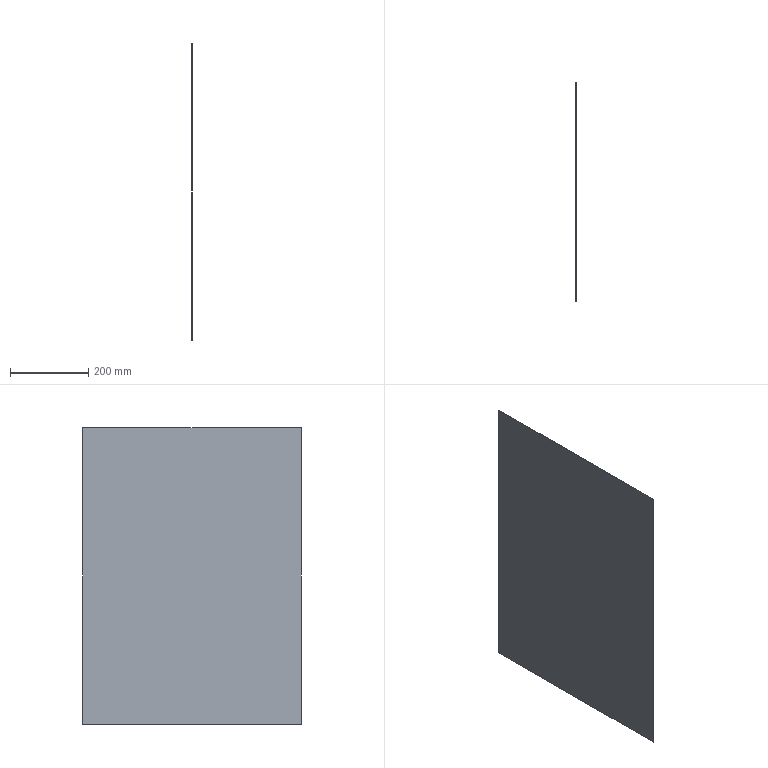Part | SolidWorks | 1 solid | 6 faces | box 1.5 x 560 x 759 mm | volume 637560 mm3 | plane 6
STEP:
#1=CARTESIAN_POINT('',(0.,280.,379.5));
#2=VERTEX_POINT('',#1);
#3=CARTESIAN_POINT('',(0.,-280.,379.5));
#4=VERTEX_POINT('',#3);
#5=CARTESIAN_POINT('',(0.,-280.,379.5));
#6=DIRECTION('',(0.,-1.,0.));
#7=VECTOR('',#6,1000.);
#8=LINE('',#5,#7);
#9=EDGE_CURVE('',#2,#4,#8,.T.);
#10=ORIENTED_EDGE('',*,*,#9,.F.);
#11=CARTESIAN_POINT('',(-1.5,280.,379.5));
#12=VERTEX_POINT('',#11);
#13=CARTESIAN_POINT('',(-1.5,280.,379.5));
#14=DIRECTION('',(1.,0.,0.));
#15=VECTOR('',#14,1000.);
#16=LINE('',#13,#15);
#17=EDGE_CURVE('',#12,#2,#16,.T.);
#18=ORIENTED_EDGE('',*,*,#17,.F.);
#19=CARTESIAN_POINT('',(-1.5,-280.,379.5));
#20=VERTEX_POINT('',#19);
#21=CARTESIAN_POINT('',(-1.5,-280.,379.5));
#22=DIRECTION('',(0.,-1.,0.));
#23=VECTOR('',#22,1000.);
#24=LINE('',#21,#23);
#25=EDGE_CURVE('',#12,#20,#24,.T.);
#26=ORIENTED_EDGE('',*,*,#25,.T.);
#27=CARTESIAN_POINT('',(-1.5,-280.,379.5));
#28=DIRECTION('',(1.,0.,0.));
#29=VECTOR('',#28,1000.);
#30=LINE('',#27,#29);
#31=EDGE_CURVE('',#20,#4,#30,.T.);
#32=ORIENTED_EDGE('',*,*,#31,.T.);
#33=EDGE_LOOP('',(#10,#18,#26,#32));
#34=FACE_OUTER_BOUND('',#33,.T.);
#35=CARTESIAN_POINT('',(-1.5,-280.,379.5));
#36=DIRECTION('',(0.,0.,1.));
#37=DIRECTION('',(1.,0.,0.));
#38=AXIS2_PLACEMENT_3D('',#35,#36,#37);
#39=PLANE('',#38);
#40=ADVANCED_FACE('',(#34),#39,.T.);
#41=CARTESIAN_POINT('',(0.,280.,-379.5));
#42=VERTEX_POINT('',#41);
#43=CARTESIAN_POINT('',(0.,280.,-379.5));
#44=DIRECTION('',(0.,0.,1.));
#45=VECTOR('',#44,1000.);
#46=LINE('',#43,#45);
#47=EDGE_CURVE('',#42,#2,#46,.T.);
#48=ORIENTED_EDGE('',*,*,#47,.F.);
#49=CARTESIAN_POINT('',(-1.5,280.,-379.5));
#50=VERTEX_POINT('',#49);
#51=CARTESIAN_POINT('',(-1.5,280.,-379.5));
#52=DIRECTION('',(1.,0.,0.));
#53=VECTOR('',#52,1000.);
#54=LINE('',#51,#53);
#55=EDGE_CURVE('',#50,#42,#54,.T.);
#56=ORIENTED_EDGE('',*,*,#55,.F.);
#57=CARTESIAN_POINT('',(-1.5,280.,-379.5));
#58=DIRECTION('',(0.,0.,1.));
#59=VECTOR('',#58,1000.);
#60=LINE('',#57,#59);
#61=EDGE_CURVE('',#50,#12,#60,.T.);
#62=ORIENTED_EDGE('',*,*,#61,.T.);
#63=ORIENTED_EDGE('',*,*,#17,.T.);
#64=EDGE_LOOP('',(#48,#56,#62,#63));
#65=FACE_OUTER_BOUND('',#64,.T.);
#66=CARTESIAN_POINT('',(-1.5,280.,-379.5));
#67=DIRECTION('',(0.,1.,0.));
#68=DIRECTION('',(0.,0.,1.));
#69=AXIS2_PLACEMENT_3D('',#66,#67,#68);
#70=PLANE('',#69);
#71=ADVANCED_FACE('',(#65),#70,.T.);
#72=CARTESIAN_POINT('',(0.,-280.,-379.5));
#73=VERTEX_POINT('',#72);
#74=CARTESIAN_POINT('',(0.,-280.,-379.5));
#75=DIRECTION('',(0.,1.,0.));
#76=VECTOR('',#75,1000.);
#77=LINE('',#74,#76);
#78=EDGE_CURVE('',#73,#42,#77,.T.);
#79=ORIENTED_EDGE('',*,*,#78,.F.);
#80=CARTESIAN_POINT('',(-1.5,-280.,-379.5));
#81=VERTEX_POINT('',#80);
#82=CARTESIAN_POINT('',(-1.5,-280.,-379.5));
#83=DIRECTION('',(1.,0.,0.));
#84=VECTOR('',#83,1000.);
#85=LINE('',#82,#84);
#86=EDGE_CURVE('',#81,#73,#85,.T.);
#87=ORIENTED_EDGE('',*,*,#86,.F.);
#88=CARTESIAN_POINT('',(-1.5,-280.,-379.5));
#89=DIRECTION('',(0.,1.,0.));
#90=VECTOR('',#89,1000.);
#91=LINE('',#88,#90);
#92=EDGE_CURVE('',#81,#50,#91,.T.);
#93=ORIENTED_EDGE('',*,*,#92,.T.);
#94=ORIENTED_EDGE('',*,*,#55,.T.);
#95=EDGE_LOOP('',(#79,#87,#93,#94));
#96=FACE_OUTER_BOUND('',#95,.T.);
#97=CARTESIAN_POINT('',(-1.5,-280.,-379.5));
#98=DIRECTION('',(0.,0.,-1.));
#99=DIRECTION('',(-1.,0.,0.));
#100=AXIS2_PLACEMENT_3D('',#97,#98,#99);
#101=PLANE('',#100);
#102=ADVANCED_FACE('',(#96),#101,.T.);
#103=CARTESIAN_POINT('',(0.,-280.,-379.5));
#104=DIRECTION('',(0.,0.,-1.));
#105=VECTOR('',#104,1000.);
#106=LINE('',#103,#105);
#107=EDGE_CURVE('',#4,#73,#106,.T.);
#108=ORIENTED_EDGE('',*,*,#107,.F.);
#109=ORIENTED_EDGE('',*,*,#31,.F.);
#110=CARTESIAN_POINT('',(-1.5,-280.,-379.5));
#111=DIRECTION('',(0.,0.,-1.));
#112=VECTOR('',#111,1000.);
#113=LINE('',#110,#112);
#114=EDGE_CURVE('',#20,#81,#113,.T.);
#115=ORIENTED_EDGE('',*,*,#114,.T.);
#116=ORIENTED_EDGE('',*,*,#86,.T.);
#117=EDGE_LOOP('',(#108,#109,#115,#116));
#118=FACE_OUTER_BOUND('',#117,.T.);
#119=CARTESIAN_POINT('',(-1.5,-280.,-379.5));
#120=DIRECTION('',(0.,-1.,0.));
#121=DIRECTION('',(0.,0.,-1.));
#122=AXIS2_PLACEMENT_3D('',#119,#120,#121);
#123=PLANE('',#122);
#124=ADVANCED_FACE('',(#118),#123,.T.);
#125=ORIENTED_EDGE('',*,*,#25,.F.);
#126=ORIENTED_EDGE('',*,*,#61,.F.);
#127=ORIENTED_EDGE('',*,*,#92,.F.);
#128=ORIENTED_EDGE('',*,*,#114,.F.);
#129=EDGE_LOOP('',(#125,#126,#127,#128));
#130=FACE_OUTER_BOUND('',#129,.T.);
#131=CARTESIAN_POINT('',(-1.5,0.,0.));
#132=DIRECTION('',(1.,0.,0.));
#133=DIRECTION('',(0.,0.,-1.));
#134=AXIS2_PLACEMENT_3D('',#131,#132,#133);
#135=PLANE('',#134);
#136=ADVANCED_FACE('',(#130),#135,.F.);
#137=ORIENTED_EDGE('',*,*,#9,.T.);
#138=ORIENTED_EDGE('',*,*,#107,.T.);
#139=ORIENTED_EDGE('',*,*,#78,.T.);
#140=ORIENTED_EDGE('',*,*,#47,.T.);
#141=EDGE_LOOP('',(#137,#138,#139,#140));
#142=FACE_OUTER_BOUND('',#141,.T.);
#143=CARTESIAN_POINT('',(0.,0.,0.));
#144=DIRECTION('',(1.,0.,0.));
#145=DIRECTION('',(0.,0.,-1.));
#146=AXIS2_PLACEMENT_3D('',#143,#144,#145);
#147=PLANE('',#146);
#148=ADVANCED_FACE('',(#142),#147,.T.);
#149=CLOSED_SHELL('',(#40,#71,#102,#124,#136,#148));
#150=MANIFOLD_SOLID_BREP('',#149);
#151=CARTESIAN_POINT('',(0.,0.,0.));
#152=DIRECTION('',(0.,0.,1.));
#153=DIRECTION('',(1.,0.,0.));
#154=AXIS2_PLACEMENT_3D('',#151,#152,#153);
#155=(LENGTH_UNIT()NAMED_UNIT(*)SI_UNIT(.MILLI.,.METRE.));
#156=UNCERTAINTY_MEASURE_WITH_UNIT(LENGTH_MEASURE(0.00001),#155,'','');
#157=(NAMED_UNIT(*)PLANE_ANGLE_UNIT()SI_UNIT($,.RADIAN.));
#158=(NAMED_UNIT(*)SI_UNIT($,.STERADIAN.)SOLID_ANGLE_UNIT());
#159=(GEOMETRIC_REPRESENTATION_CONTEXT(3)GLOBAL_UNCERTAINTY_ASSIGNED_CONTEXT((#156))GLOBAL_UNIT_ASSIGNED_CONTEXT((#155,#157,#158))REPRESENTATION_CONTEXT('',''));
#160=ADVANCED_BREP_SHAPE_REPRESENTATION('',(#150,#154),#159);